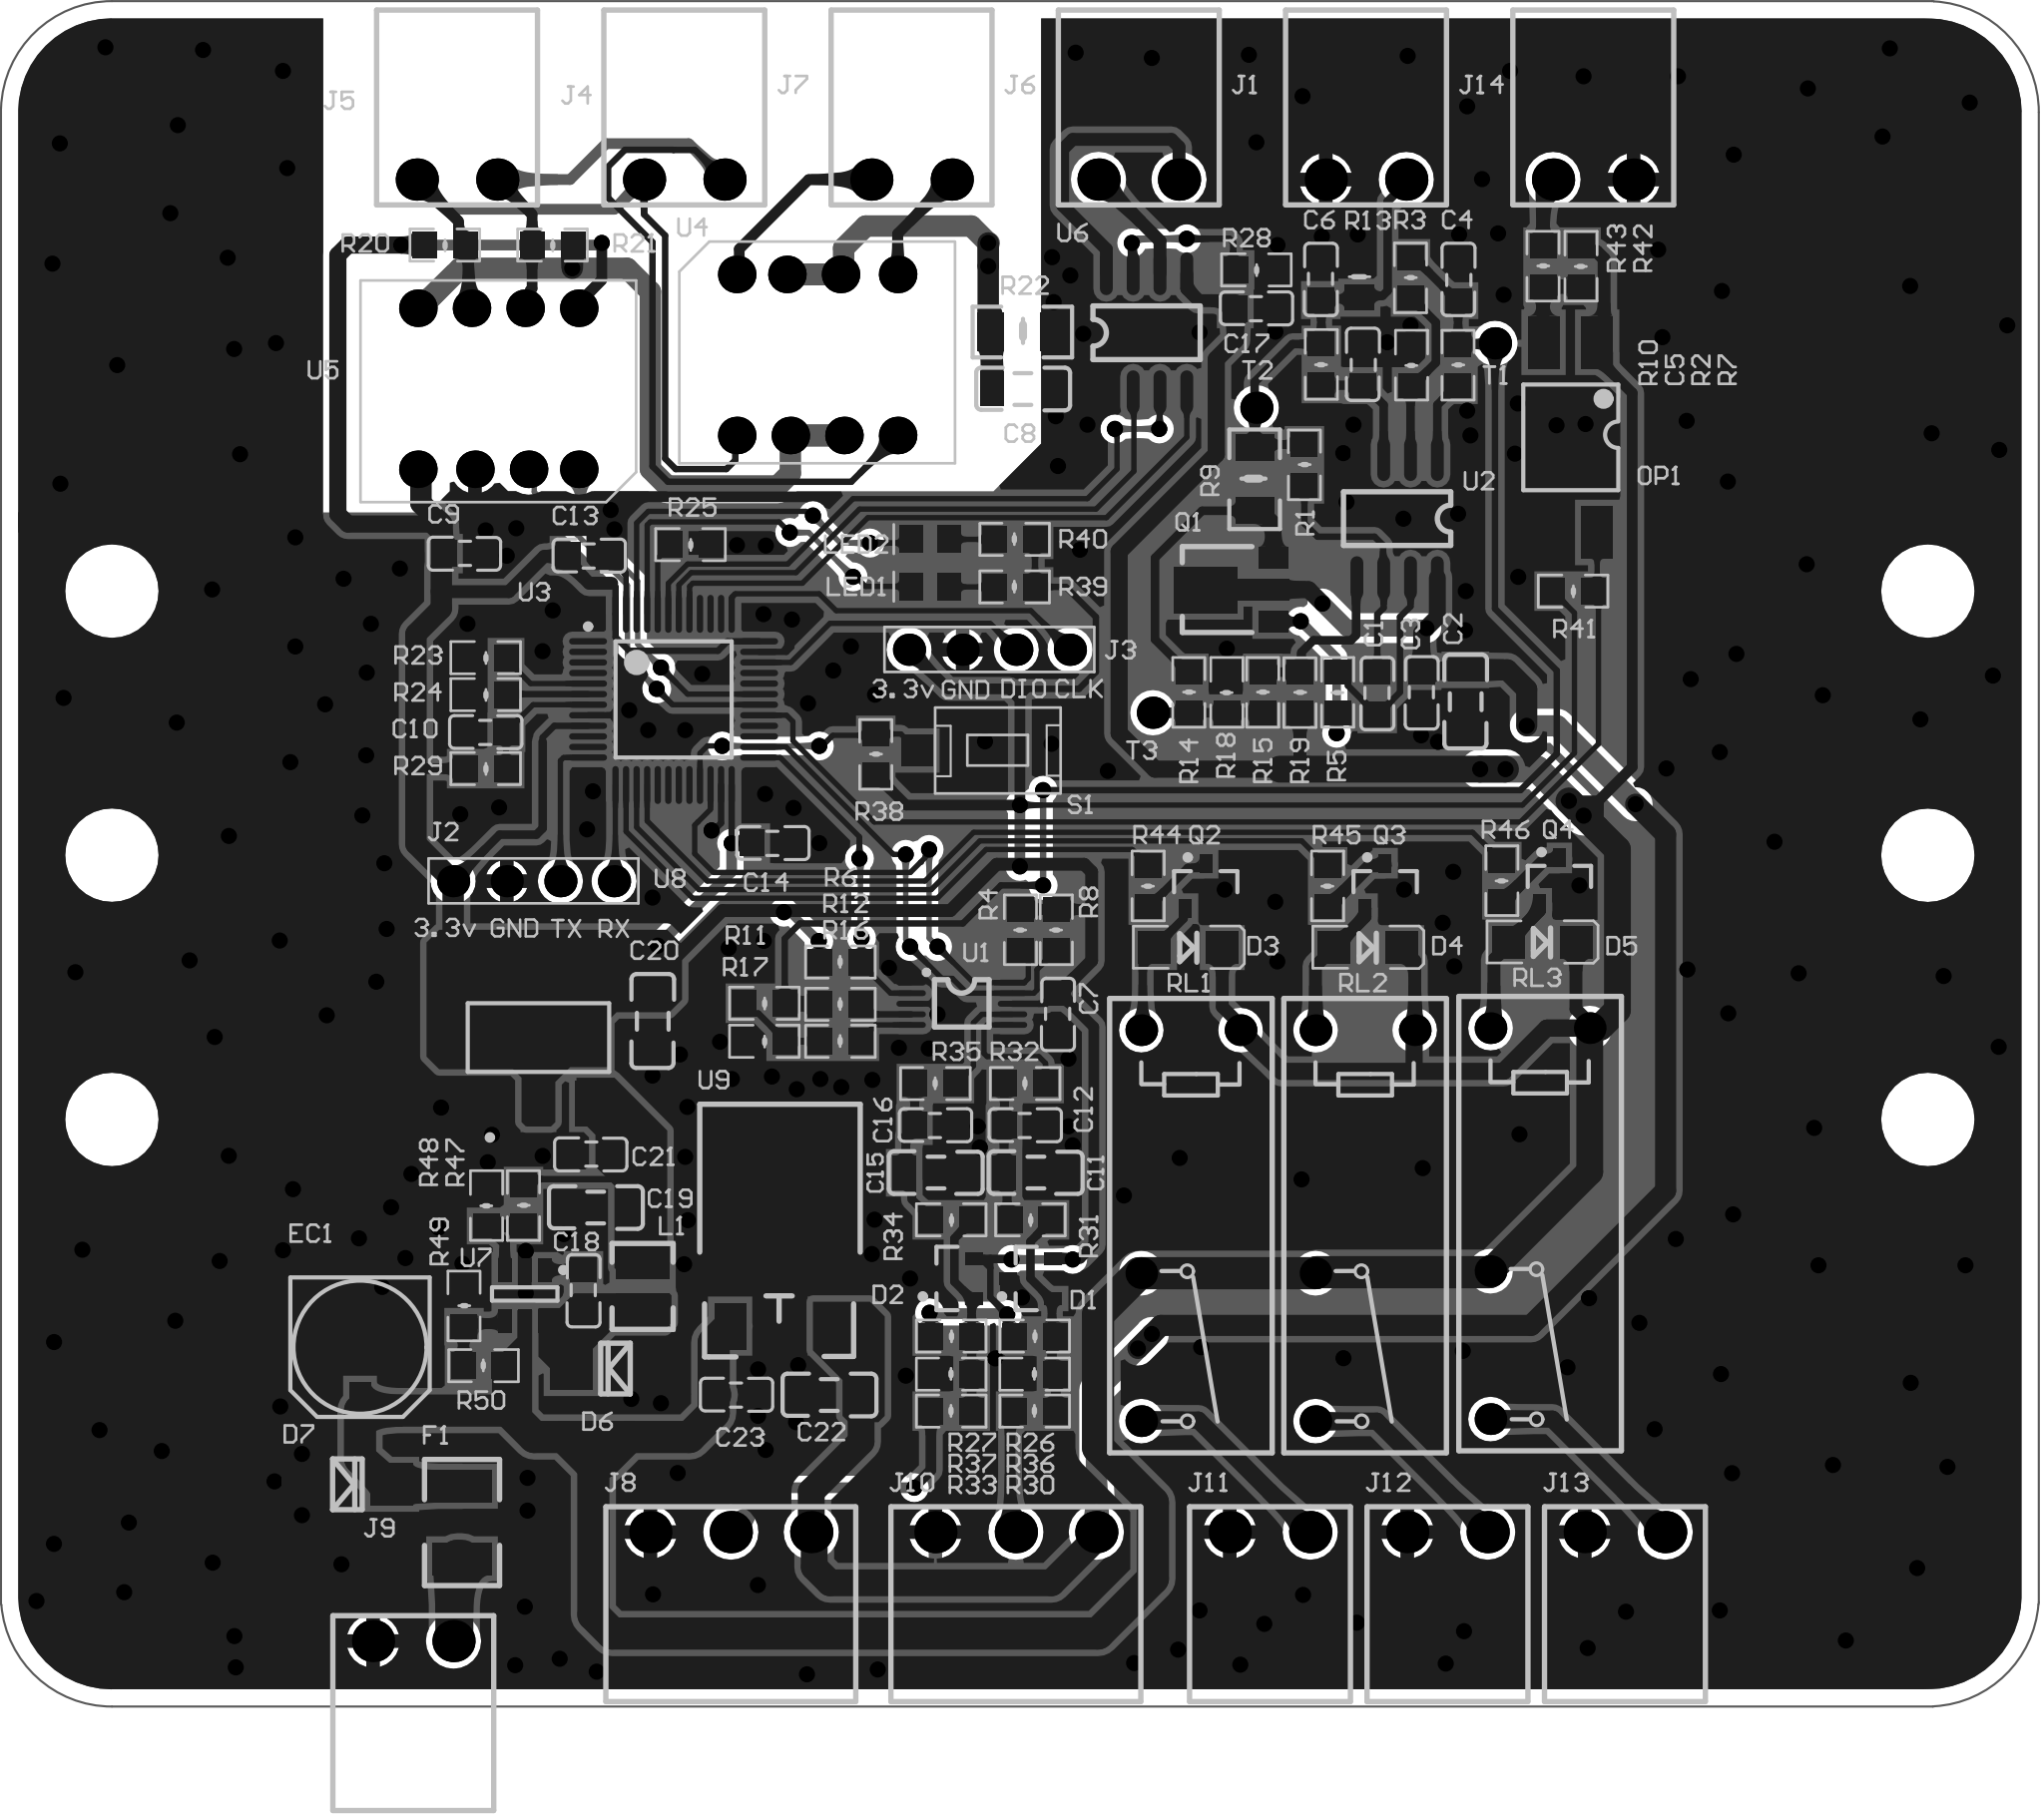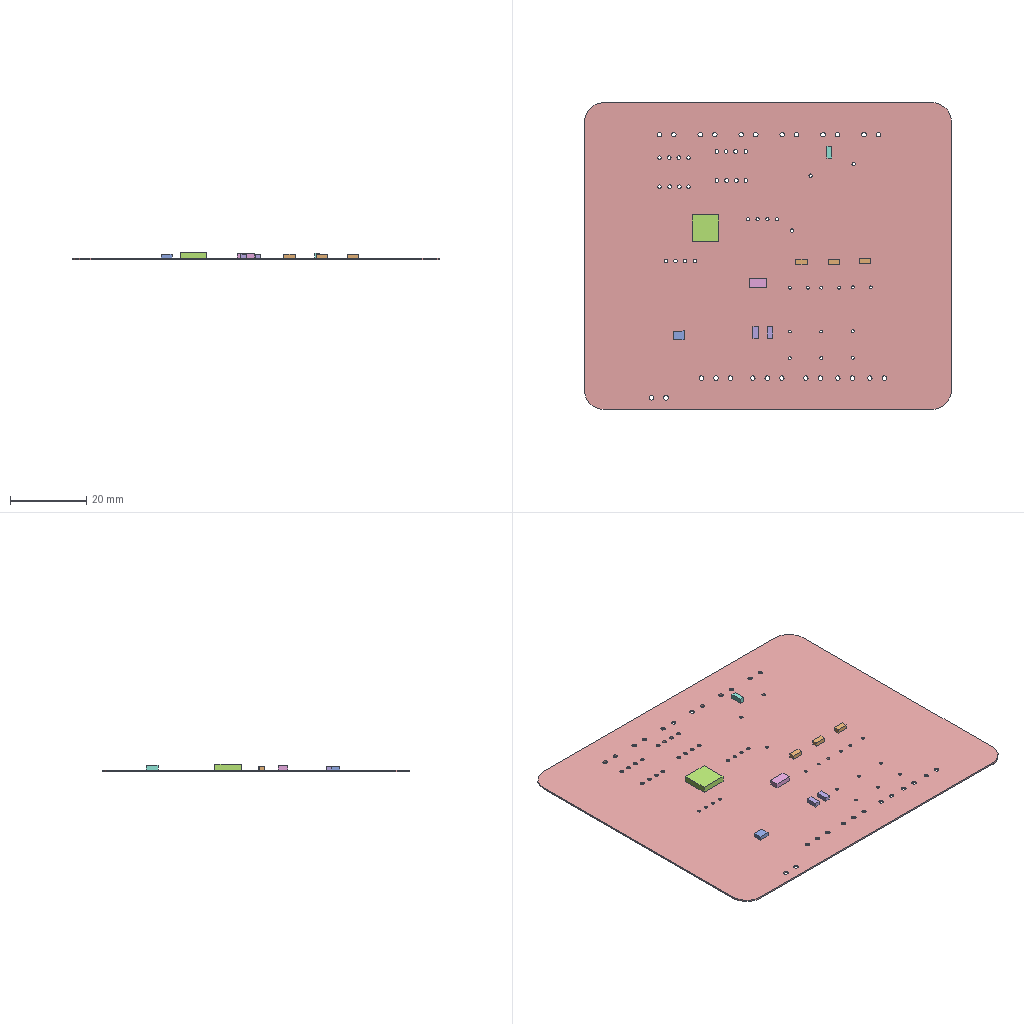Circuit board layout | Altium Designer | box 96.5 x 80.7 x 2 mm
Layer stack:
# Altium Designer layer stack of  (unit mm; dielectric type: 0 none, 1 core, 2 prepreg, 3 surface material)
index,name,kind,layer,copper_thickness_mm,dielectric_type,dielectric_thickness_mm,dielectric_material,dielectric_constant
0,Top Paste,other,,,,,,
1,Top Overlay,other,,,,,,
2,Top Solder,dielectric,,,3,0.0102,Solder Resist,3.5
3,Top Layer,copper,Top Layer,0.0356,,,,
4,Dielectric 1,dielectric,,,0,0.32,FR-4,4.8
5,Bottom Layer,copper,Bottom Layer,0.0356,,,,
6,Bottom Solder,dielectric,,,3,0.0102,Solder Resist,3.5
7,Bottom Overlay,other,,,,,,
8,Bottom Paste,other,,,,,,
# drill layer pairs: low layer,high layer
drill_pair,Top Layer,Bottom Layer
Part placement:
Designator,Comment,Layer,Footprint,Center-X(mm),Center-Y(mm),Rotation
C21,104,TopLayer,0805-C-I,-20.309,25.875,0
C20,10uf,TopLayer,1206-C-I,-17.4,32.19,90
U9,7812,TopLayer,TO-252,-11.361,21.246,0
U8,AMS1117-3.3,TopLayer,SOT-223_-_3,-22.8,31.4,0
U7,MP2451,TopLayer,SOT23-6,-23.45,19.2,270
U6,DRV8872,TopLayer,SOP8-9,6,64.75,90
U5,ZLG-RSM485M,TopLayer,ZLG-RSM485M,-24.7,62.1,180
U4,ZLG-SP00S12,TopLayer,ZLG-SP00S12,-9.6,63.7,0
U3,GD32F103C8T6,TopLayer,LQFP48_N,-16.4,47.4,0
U2,TL1490,TopLayer,SO-8,17.865,55.956,270
U1,ADS1115,TopLayer,MSOP-10,-2.75,33,0
T3,,TopLayer,TP-TEST,6.3,46.77,0
T2,,TopLayer,TP-TEST,11.2,61.2,0
T1,,TopLayer,TP-TEST,22.5,64.25,0
S1,SW,TopLayer,KEY-3*6,-1.041,44.983,180
RL3,HF-46F,TopLayer,RY-HF46F,24.638,22.597,180
RL2,HF-46F,TopLayer,RY-HF46F,16.35,22.5,180
RL1,HF-46F,TopLayer,RY-HF46F,8.1,22.5,180
R50,124k,TopLayer,0805-R-I,-25.4,15.875,0
R49,24K,TopLayer,0805-R-I,-26.325,18.7,270
R48,20K,TopLayer,0805-R-I,-25.258,23.451,90
R47,124K,TopLayer,0805-R-I,-23.508,23.451,270
R46,4.7k,TopLayer,0805-R-I,22.825,38.825,90
R45,4.7k,TopLayer,0805-R-I,14.575,38.575,90
R44,4.7k,TopLayer,0805-R-I,6.075,38.575,90
R43,4.7k,TopLayer,0805-R-I,24.775,67.9,270
R42,1k,TopLayer,0805-R-I,26.575,67.9,90
R41,4.7k,TopLayer,0805-R-I,26.2,52.525,180
R40,10k,TopLayer,0805-R-I,-0.25,54.975,0
R39,10k,TopLayer,0805-R-I,-0.25,52.725,0
R38,10k,TopLayer,0805-R-I,-6.825,44.8,270
R37,30k,TopLayer,0805-R-I,-3.25,15.475,0
R36,30k,TopLayer,0805-R-I,0.7,15.475,0
R35,0,TopLayer,0805-R-I,-4,29.225,0
R34,1k,TopLayer,0805-R-I,-3.25,22.775,180
R33,100k,TopLayer,0805-R-I,-3.25,13.725,0
R32,0,TopLayer,0805-R-I,0.25,29.225,0
R31,1k,TopLayer,0805-R-I,0.5,22.775,180
R30,100k,TopLayer,0805-R-I,0.7,13.725,0
R29,10k,TopLayer,0805-R-I,-25.3,44.125,180
R28,0.15R,TopLayer,0805-R-I,11.2,67.725,180
R27,1M,TopLayer,0805-R-I,-3.25,17.275,180
R26,1M,TopLayer,0805-R-I,0.7,17.275,180
R25,10k,TopLayer,0805-R-I,-15.6,54.725,180
R24,10k,TopLayer,0805-R-I,-25.3,47.625,180
R23,10k,TopLayer,0805-R-I,-25.3,49.375,180
R22,1M,TopLayer,1206-R-I,0.1176,64.783,0
R21,10k,TopLayer,0805-R-I,-22.135,68.9,180
R20,10k,TopLayer,0805-R-I,-27.235,68.9,180
R19,2004/NC,TopLayer,0805-R-I,13.263,47.722,270
R18,1201,TopLayer,0805-R-I,9.801,47.735,90
R17,10k,TopLayer,0805-R-I,-12.1,31.225,180
R16,0,TopLayer,0805-R-I,-8.5,31.225,0
R15,4.7k,TopLayer,0805-R-I,11.5,47.735,270
R14,9100,TopLayer,0805-R-I,8,47.735,270
R13,,TopLayer,R[0805],16.075,67.4,270
R12,0,TopLayer,0805-R-I,-8.5,32.975,0
R11,10k,TopLayer,0805-R-I,-12.1,33.025,180
R10,1k,TopLayer,0805-R-I,14.275,63.25,90
R9,100,TopLayer,1206-R-I,11.117,57.818,90
R8,10k,TopLayer,0805-R-I,1.725,36.5,90
R7,1k,TopLayer,0805-R-I,20.75,63.215,270
R6,10k,TopLayer,0805-R-I,-8.5,34.975,0
R5,100R,TopLayer,0805-R-I,15.051,47.735,90
R4,10k,TopLayer,0805-R-I,0.0254,36.5,90
R3,30k,TopLayer,0805-R-I,18.5,67.347,270
R2,10k,TopLayer,0805-R-I,18.551,63.215,90
R1,4.7k,TopLayer,0805-R-I,13.475,58.5,270
Q4,S8050,TopLayer,SOT23_L,25.55,38.825,90
Q3,S8050,TopLayer,SOT23_L,17.3,38.575,90
Q2,S8050,TopLayer,SOT23_L,8.8,38.575,90
Q1,S8050,TopLayer,SOT-89-3-1,10.4,52.6,90
OP1,EL817,TopLayer,EL-817,26.07,59.8,270
LED2,0805,TopLayer,LED[0805],-4.25,55,0
LED1,0805,TopLayer,LED[0805],-4.25,52.75,0
L1,4.7UH,TopLayer,L-252012,-17.868,19.625,90
J14,KF2EDG-3.81-2P,TopLayer,3.81-2P-90,27.155,72,180
J13,KF2EDG-3.81-2P,TopLayer,3.81-2P-90,28.655,8,0
J12,KF2EDG-3.81-2P,TopLayer,3.81-2P-90,20.25,8,0
J11,KF2EDG-3.81-2P,TopLayer,3.81-2P-90,11.845,8,0
J10,KF2EDG-3.81-3P,TopLayer,3.81-3P-90,-0.19,8,0
J9,KF2EDG-3.81-2P,TopLayer,3.81-2P-90,-28.727,2.845,0
J8,KF2EDG-3.81-3P,TopLayer,3.81-3P-90,-13.69,8,0
J7,KF2EDG-3.81-2P,TopLayer,3.81-2P-90,-5.131,72,180
J6,KF2EDG-3.81-2P,TopLayer,3.81-2P-90,5.631,72,180
J5,KF2EDG-3.81-2P,TopLayer,3.81-2P-90,-26.655,72,180
J4,KF2EDG-3.81-2P,TopLayer,3.81-2P-90,-15.893,72,180
J3,xh2.54,TopLayer,CON4,-1.44,49.75,180
J2,xh2.54,TopLayer,CON4,-23.03,38.8,180
J1,Sensor,TopLayer,3.81-2P-90,16.393,72,180
F1,PPTC,TopLayer,1210-F,-26.419,8.453,90
EC1,100UF,TopLayer,C6.3X6.3,-31.25,16.75,90
D7,SS34,TopLayer,DO-SMA-I,-31.848,10.262,180
D6,SS34,TopLayer,DO-SMA-I,-19.152,15.738,0
D5,4148,TopLayer,D1206,24.731,35.906,0
D4,4148,TopLayer,D1206,16.481,35.656,0
D3,4148,TopLayer,D1206,7.981,35.656,0
D2,BTA54S,TopLayer,SOT23_L,-3.25,20,180
D1,BTA54S,TopLayer,SOT23_L,0.5,20,180
C23,104,TopLayer,0805-C-I,-13.432,14.496,180
C22,22uf,TopLayer,1206-C-I,-9.01,14.5,0
C19,22uf,TopLayer,1206-C-I,-20.073,23.37,0
C18,104,TopLayer,0805-C-I,-20.668,19.435,90
C17,104,TopLayer,0805-C-I,11.191,65.9,180
C16,104,TopLayer,0805-C-I,-4.009,27.25,180
C15,NC,TopLayer,1206-C-I,-3.99,25,180
C14,104,TopLayer,0805-C-I,-11.709,40.6,180
C13,104,TopLayer,0805-C-I,-20.409,54.2,180
C12,104,TopLayer,0805-C-I,0.2406,27.25,180
C11,NC,TopLayer,1206-C-I,0.74,25,180
C10,104,TopLayer,0805-C-I,-25.309,45.85,180
C9,104,TopLayer,0805-C-I,-26.291,54.3,0
C8,102-2KV,TopLayer,1206-C-I,0.16,62.1,0
C7,104,TopLayer,0805-C-I,1.8,32.509,90
C6,104,TopLayer,0805-C-I,14.25,67.286,90
C5,104,TopLayer,0805-C-I,16.25,63.241,270
C4,104,TopLayer,0805-C-I,20.775,67.259,270
C3,104,TopLayer,0805-C-I,19.025,47.725,90
C2,10uf,TopLayer,1206-C-I,21.1,47.31,90
C1,104,TopLayer,0805-C-I,16.925,47.691,90
Pad and via stacks:
# Altium Designer via and pad stacks of  (unit mm). Each distinct definition once, with the count of objects using it.
# via: kind,start_layer,end_layer,hole_mm,diameter_mm,mode(0 simple;1 top-mid-bottom;2 full stack),diameter_per_layer,count,example_net
# pad: kind,layer,hole_mm,hole_type(0 round;1 square;2 slot),plating,top_size,top_shape(1 round;2 rect;3 octagon;9 rounded rect),mid_size,bottom_size,mode,footprint,size_per_layer,count,example
pad,Top Layer,0,0,plated,1.143x1.27,2,1.143x1.27,1.143x1.27,0,0805-R-I,,94,R38.2
pad,Top Layer,0,0,plated,1.1x2.15,2,1.1x2.15,1.1x2.15,0,SOT-223 - 3,,3,U8.1
pad,Top Layer,0,0,plated,3.5x2.15,2,3.5x2.15,3.5x2.15,0,SOT-223 - 3,,1,U8.2
pad,Top Layer,0,0,plated,0.28x1.4,1,0.28x1.4,0.28x1.4,0,MSOP-10,,10,U1.1
pad,Top Layer,0,0,plated,1.143x1.27,2,1.143x1.27,1.143x1.27,0,0805-C-I,,16,C16.2
pad,Top Layer,0,0,plated,1.2x1.27,2,1.2x1.27,1.2x1.27,0,0805-C-I,,16,C16.1
pad,Top Layer,0,0,plated,1.13x1.651,2,1.13x1.651,1.13x1.651,0,1206-C-I,,14,C15.1
pad,Top Layer,0,0,plated,0.6x0.85,2,0.6x0.85,0.6x0.85,0,SOT23_L,,15,D2.3
pad,Top Layer,0,0,plated,2.5x1.5,2,2.5x1.5,2.5x1.5,0,EL-817,,4,OP1.4
pad,Top Layer,0,0,plated,1.524x2.54,2,1.524x2.54,1.524x2.54,0,L-252012,,2,L1.1
pad,Top Layer,0,0,plated,2x2,2,2x2,2x2,0,DO-SMA-I,,4,D6.2
pad,Top Layer,0,0,plated,0.65x1.1,2,0.65x1.1,0.65x1.1,0,SOT23-6,,6,U7.1
pad,Top Layer,0,0,plated,1.5x1.5,2,1.5x1.5,1.5x1.5,0,KEY-3*6,,2,S1.2
pad,Top Layer,0,0,plated,0.3x1.8,1,0.3x1.8,0.3x1.8,0,LQFP48_N,,48,U3.1
pad,Top Layer,0,0,plated,1.3x1.1,2,1.3x1.1,1.3x1.1,0,LED[0805],,4,LED2.2
pad,Top Layer,0,0,plated,1.524x1.524,2,1.524x1.524,1.524x1.524,0,D1206,,6,D4.2
pad,Top Layer,0,0,plated,2.032x0.6096,1,2.032x0.6096,2.032x0.6096,0,SO-8,,8,U2.8
pad,Top Layer,0,0,plated,1.27x1.8,2,1.27x1.8,1.27x1.8,0,1206-R-I,,4,R9.2
pad,Top Layer,0,0,plated,2.3x2.3,2,2.3x2.3,2.3x2.3,0,SOP8-9,,1,U6.9
pad,Top Layer,0,0,plated,2.032x0.6096,1,2.032x0.6096,2.032x0.6096,0,SOP8-9,,8,U6.8
pad,Top Layer,0,0,plated,1.397x1.2,2,1.397x1.2,1.397x1.2,0,R[0805],,2,R13.2
pad,Top Layer,0,0,plated,1.016x1.397,2,1.016x1.397,1.016x1.397,0,SOT-89-3-1,,2,Q1.1
pad,Top Layer,0,0,plated,1.016x2.8,2,1.016x2.8,1.016x2.8,0,SOT-89-3-1,,1,Q1.3
pad,Top Layer,0,0,plated,2.2x3,2,2.2x3,2.2x3,0,SOT-89-3-1,,1,Q1.3
pad,Top Layer,0,0,plated,1.524x2.794,2,1.524x2.794,1.524x2.794,0,1210-F,,2,F1.2
pad,Top Layer,0,0,plated,7x6.5,2,7x6.5,7x6.5,0,TO-252,,1,U9.2
pad,Top Layer,0,0,plated,1.5x2.2,2,1.5x2.2,1.5x2.2,0,TO-252,,2,U9.1
pad,Top Layer,0,0,plated,2.7x1,2,2.7x1,2.7x1,0,C6.3X6.3,,2,EC1.1
pad,Multi-Layer,1.2,0,plated,2x2,1,2x2,2x2,0,3.81-2P-90,,20,J9.1
pad,Multi-Layer,0.889,0,plated,1.524x1.524,1,1.524x1.524,1.524x1.524,0,TP-TEST,,3,T3.1
pad,Multi-Layer,0.889,0,plated,1.524x1.524,1,1.524x1.524,1.524x1.524,0,CON4,,6,J3.4
pad,Multi-Layer,0.889,0,plated,1.524x1.524,1,1.524x1.524,1.524x1.524,1,CON4,,2,J3.3
pad,Multi-Layer,0.75,0,plated,1.5x1.5,1,1.5x1.5,1.5x1.5,0,RY-HF46F,,12,RL1.2
pad,Multi-Layer,1.016,0,plated,1.778x1.778,1,1.778x1.778,1.778x1.778,0,ZLG-SP00S12,,8,U4.1
pad,Multi-Layer,1.016,0,plated,1.778x1.778,1,1.778x1.778,1.778x1.778,0,ZLG-RSM485M,,8,U5.1
pad,Multi-Layer,1.2,0,plated,2x2,1,2x2,2x2,0,3.81-3P-90,,6,J8.3
via,Top Layer,Bottom Layer,0.4064,0.762,0,,317,ADS-AD2
Copper pours:
name,layer,net,type(0 solid;1 hatched;2 none)
GND_L02_P000,Bottom Layer,GND,0
GND_L02_P003,Bottom Layer,GND,0
GND_L01_P001,Top Layer,GND,0
GND_L01_P004,Top Layer,GND,0
Design rules, without the lines most boards share:
# Altium Designer design rules of  (exported by Altium Designer, unit mm)
# columns: name | kind | enabled | priority | scope1 | scope2 | descriptor | typed fields (field=value)
NetAntennae | 56 | enabled | 1 | All | All | Net Antennae (Tolerance=0mm) (All) |
SilkToSilkClearance | 55 | enabled | 1 | All | All | Silk to Silk (Clearance=0.254mm) (All),(All) |
SilkToSolderMaskClearance | 54 | enabled | 1 | IsPad | All | Silk To Solder Mask (Clearance=0.254mm) (IsPad),(All) |
MinimumSolderMaskSliver | 53 | enabled | 1 | All | All | Minimum Solder Mask Sliver (Gap=0.254mm) (All),(All) |
HoleToHoleClearance | 52 | enabled | 1 | All | All | Hole To Hole Clearance (Gap=0.254mm) (All),(All) | gap=0.254
DiffPairsRouting | 51 | enabled | 1 | All | All | Differential Pairs Uncoupled Length using the Gap Constraints (Min=0.254mm) (Max=0.254mm) (Prefered=0.254mm)  and Width Constraints (Min=0.381mm) (Max=0.381mm) (Prefered=0.381mm) (All) |
HoleSize | 42 | enabled | 1 | All | All | Hole Size Constraint (Min=0.025mm) (Max=2.54mm) (All) |
Height | 50 | enabled | 1 | All | All | Height Constraint (Min=0mm) (Max=254mm) (Prefered=12.7mm) (All) | min_height=0 max_height=254
ComponentClearance | 24 | enabled | 1 | All | All | Component Clearance Constraint ( Horizontal Gap = 0.254mm, Vertical Gap = 0.254mm ) (All),(All)  | gap=0.254
SolderMaskExpansion | 13 | enabled | 1 | All | All | Solder Mask Expansion (Expansion =0mm) (All) | expansion=0
PasteMaskExpansion | 14 | enabled | 1 | All | All | Paste Mask Expansion (Expansion =0mm) (All) | expansion=0
RoutingVias | 11 | enabled | 1 | All | All | Routing Via (MinHoleWidth=0.305mm) (MaxHoleWidth=0.711mm) (PreferredHoleWidth=0.711mm) (MinWidth=0.508mm) (MaxWidth=1.27mm) (PreferedWidth=1.27mm) (All) | via_min_hole=0.3048 via_max_hole=0.7112 via_preferred_diameter=1.27 via_preferred_hole=0.7112
RoutingCorners | 10 | enabled | 1 | All | All | Routing Corners (Style=45-Degree) (Min Setback=2.54mm) (Max Setback=2.54mm) (All) |
Width | 2 | enabled | 1 | All | All | Width Constraint (Min=0.254mm) (Max=2.54mm) (Preferred=0.254mm) (All) |
PolygonConnect | 20 | enabled | 1 | All | All | Polygon Connect Rule(Relief Connect )(Conductor Width=0.635mm) (Relief Angle=90 Angle) (Entries=4) (Air Gap Width=0.254mm) (All),(All) | connect_style(0=relief,1=direct,2=none)=0 relief_conductor_width=0.635 relief_entries=4
PlaneClearance | 12 | enabled | 1 | All | All | Power Plane Clearance (Clearance =0.508mm) (All) | clearance=0.508
PlaneConnect | 6 | enabled | 1 | All | All | Power Plane Connect Rule(Relief Connect )(Expansion=0.508mm) (Conductor Width=0.635mm) (Air Gap=0.254mm) (Entries=4) (All) | relief_conductor_width=0.635 relief_entries=4 relief_expansion=0.508
Clearance | 0 | enabled | 2 | All | All | Clearance Constraint (Gap=0.152mm) (All),(All) | gap=0.1524
Clearance_1 | 0 | enabled | 1 | InPolygon | All | Clearance Constraint (Gap=0.508mm) (InPolygon),(All) | gap=0.508